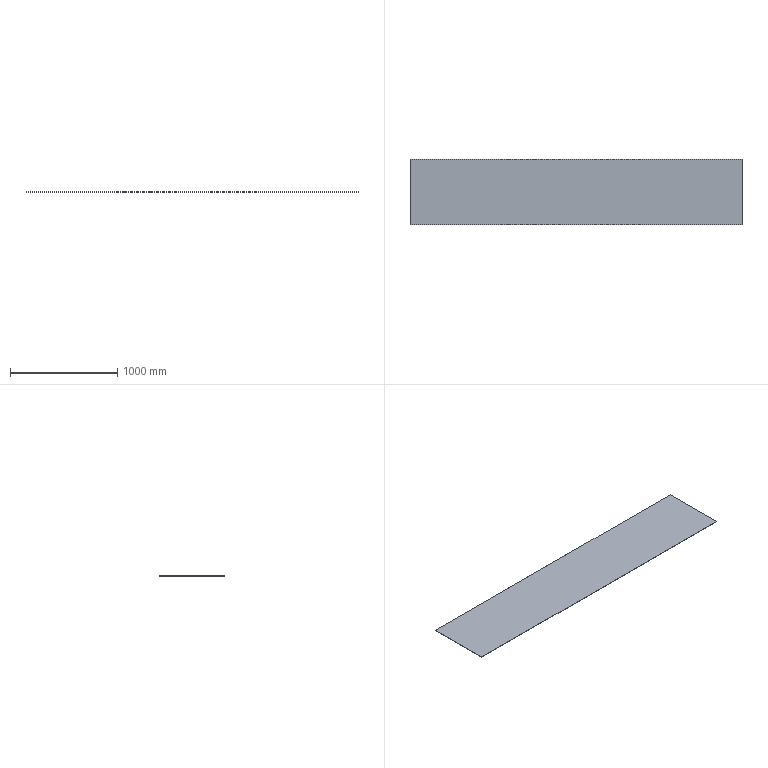Part | STEP file | 750038395 | 1 solid | 6 faces | box 3095 x 610 x 3 mm | volume 5663850 mm3 | plane 6
STEP:
#1=CARTESIAN_POINT('',(0.,-305.,3.));
#2=VERTEX_POINT('',#1);
#3=CARTESIAN_POINT('',(3095.,-305.,3.));
#4=VERTEX_POINT('',#3);
#5=CARTESIAN_POINT('',(0.,-305.,3.));
#6=DIRECTION('',(1.,0.,0.));
#7=VECTOR('',#6,1000.);
#8=LINE('',#5,#7);
#9=EDGE_CURVE('',#2,#4,#8,.T.);
#10=ORIENTED_EDGE('',*,*,#9,.T.);
#11=CARTESIAN_POINT('',(3095.,305.,3.));
#12=VERTEX_POINT('',#11);
#13=CARTESIAN_POINT('',(3095.,0.,3.));
#14=DIRECTION('',(0.,1.,0.));
#15=VECTOR('',#14,1000.);
#16=LINE('',#13,#15);
#17=EDGE_CURVE('',#4,#12,#16,.T.);
#18=ORIENTED_EDGE('',*,*,#17,.T.);
#19=CARTESIAN_POINT('',(0.,305.,3.));
#20=VERTEX_POINT('',#19);
#21=CARTESIAN_POINT('',(0.,305.,3.));
#22=DIRECTION('',(-1.,0.,0.));
#23=VECTOR('',#22,1000.);
#24=LINE('',#21,#23);
#25=EDGE_CURVE('',#12,#20,#24,.T.);
#26=ORIENTED_EDGE('',*,*,#25,.T.);
#27=CARTESIAN_POINT('',(0.,0.,3.));
#28=DIRECTION('',(0.,-1.,0.));
#29=VECTOR('',#28,1000.);
#30=LINE('',#27,#29);
#31=EDGE_CURVE('',#20,#2,#30,.T.);
#32=ORIENTED_EDGE('',*,*,#31,.T.);
#33=EDGE_LOOP('',(#10,#18,#26,#32));
#34=FACE_OUTER_BOUND('',#33,.T.);
#35=CARTESIAN_POINT('',(0.,0.,3.));
#36=DIRECTION('',(0.,0.,1.));
#37=DIRECTION('',(1.,0.,0.));
#38=AXIS2_PLACEMENT_3D('',#35,#36,#37);
#39=PLANE('',#38);
#40=ADVANCED_FACE('',(#34),#39,.T.);
#41=CARTESIAN_POINT('',(3095.,305.,0.));
#42=VERTEX_POINT('',#41);
#43=CARTESIAN_POINT('',(3095.,305.,3.));
#44=DIRECTION('',(0.,0.,-1.));
#45=VECTOR('',#44,1000.);
#46=LINE('',#43,#45);
#47=EDGE_CURVE('',#12,#42,#46,.T.);
#48=ORIENTED_EDGE('',*,*,#47,.F.);
#49=ORIENTED_EDGE('',*,*,#17,.F.);
#50=CARTESIAN_POINT('',(3095.,-305.,0.));
#51=VERTEX_POINT('',#50);
#52=CARTESIAN_POINT('',(3095.,-305.,3.));
#53=DIRECTION('',(0.,0.,1.));
#54=VECTOR('',#53,1000.);
#55=LINE('',#52,#54);
#56=EDGE_CURVE('',#51,#4,#55,.T.);
#57=ORIENTED_EDGE('',*,*,#56,.F.);
#58=CARTESIAN_POINT('',(3095.,-305.,0.));
#59=DIRECTION('',(0.,-1.,0.));
#60=VECTOR('',#59,1000.);
#61=LINE('',#58,#60);
#62=EDGE_CURVE('',#42,#51,#61,.T.);
#63=ORIENTED_EDGE('',*,*,#62,.F.);
#64=EDGE_LOOP('',(#48,#49,#57,#63));
#65=FACE_OUTER_BOUND('',#64,.T.);
#66=CARTESIAN_POINT('',(3095.,-305.,3.));
#67=DIRECTION('',(-1.,0.,0.));
#68=DIRECTION('',(0.,0.,1.));
#69=AXIS2_PLACEMENT_3D('',#66,#67,#68);
#70=PLANE('',#69);
#71=ADVANCED_FACE('',(#65),#70,.F.);
#72=ORIENTED_EDGE('',*,*,#56,.T.);
#73=ORIENTED_EDGE('',*,*,#9,.F.);
#74=CARTESIAN_POINT('',(0.,-305.,0.));
#75=VERTEX_POINT('',#74);
#76=CARTESIAN_POINT('',(0.,-305.,3.));
#77=DIRECTION('',(0.,0.,1.));
#78=VECTOR('',#77,1000.);
#79=LINE('',#76,#78);
#80=EDGE_CURVE('',#75,#2,#79,.T.);
#81=ORIENTED_EDGE('',*,*,#80,.F.);
#82=CARTESIAN_POINT('',(0.,-305.,0.));
#83=DIRECTION('',(-1.,0.,0.));
#84=VECTOR('',#83,1000.);
#85=LINE('',#82,#84);
#86=EDGE_CURVE('',#51,#75,#85,.T.);
#87=ORIENTED_EDGE('',*,*,#86,.F.);
#88=EDGE_LOOP('',(#72,#73,#81,#87));
#89=FACE_OUTER_BOUND('',#88,.T.);
#90=CARTESIAN_POINT('',(0.,-305.,3.));
#91=DIRECTION('',(0.,1.,0.));
#92=DIRECTION('',(0.,0.,1.));
#93=AXIS2_PLACEMENT_3D('',#90,#91,#92);
#94=PLANE('',#93);
#95=ADVANCED_FACE('',(#89),#94,.F.);
#96=ORIENTED_EDGE('',*,*,#80,.T.);
#97=ORIENTED_EDGE('',*,*,#31,.F.);
#98=CARTESIAN_POINT('',(0.,305.,0.));
#99=VERTEX_POINT('',#98);
#100=CARTESIAN_POINT('',(0.,305.,3.));
#101=DIRECTION('',(0.,0.,1.));
#102=VECTOR('',#101,1000.);
#103=LINE('',#100,#102);
#104=EDGE_CURVE('',#99,#20,#103,.T.);
#105=ORIENTED_EDGE('',*,*,#104,.F.);
#106=CARTESIAN_POINT('',(0.,305.,0.));
#107=DIRECTION('',(0.,1.,0.));
#108=VECTOR('',#107,1000.);
#109=LINE('',#106,#108);
#110=EDGE_CURVE('',#75,#99,#109,.T.);
#111=ORIENTED_EDGE('',*,*,#110,.F.);
#112=EDGE_LOOP('',(#96,#97,#105,#111));
#113=FACE_OUTER_BOUND('',#112,.T.);
#114=CARTESIAN_POINT('',(0.,305.,3.));
#115=DIRECTION('',(1.,0.,0.));
#116=DIRECTION('',(0.,0.,-1.));
#117=AXIS2_PLACEMENT_3D('',#114,#115,#116);
#118=PLANE('',#117);
#119=ADVANCED_FACE('',(#113),#118,.F.);
#120=ORIENTED_EDGE('',*,*,#104,.T.);
#121=ORIENTED_EDGE('',*,*,#25,.F.);
#122=ORIENTED_EDGE('',*,*,#47,.T.);
#123=CARTESIAN_POINT('',(3095.,305.,0.));
#124=DIRECTION('',(1.,0.,0.));
#125=VECTOR('',#124,1000.);
#126=LINE('',#123,#125);
#127=EDGE_CURVE('',#99,#42,#126,.T.);
#128=ORIENTED_EDGE('',*,*,#127,.F.);
#129=EDGE_LOOP('',(#120,#121,#122,#128));
#130=FACE_OUTER_BOUND('',#129,.T.);
#131=CARTESIAN_POINT('',(3095.,305.,3.));
#132=DIRECTION('',(0.,-1.,0.));
#133=DIRECTION('',(0.,0.,-1.));
#134=AXIS2_PLACEMENT_3D('',#131,#132,#133);
#135=PLANE('',#134);
#136=ADVANCED_FACE('',(#130),#135,.F.);
#137=ORIENTED_EDGE('',*,*,#62,.T.);
#138=ORIENTED_EDGE('',*,*,#86,.T.);
#139=ORIENTED_EDGE('',*,*,#110,.T.);
#140=ORIENTED_EDGE('',*,*,#127,.T.);
#141=EDGE_LOOP('',(#137,#138,#139,#140));
#142=FACE_OUTER_BOUND('',#141,.T.);
#143=CARTESIAN_POINT('',(0.,0.,0.));
#144=DIRECTION('',(0.,0.,1.));
#145=DIRECTION('',(1.,0.,0.));
#146=AXIS2_PLACEMENT_3D('',#143,#144,#145);
#147=PLANE('',#146);
#148=ADVANCED_FACE('',(#142),#147,.F.);
#149=CLOSED_SHELL('',(#40,#71,#95,#119,#136,#148));
#150=MANIFOLD_SOLID_BREP('',#149);
#151=CARTESIAN_POINT('',(0.,0.,0.));
#152=DIRECTION('',(0.,0.,1.));
#153=DIRECTION('',(1.,0.,0.));
#154=AXIS2_PLACEMENT_3D('',#151,#152,#153);
#155=(LENGTH_UNIT()NAMED_UNIT(*)SI_UNIT(.MILLI.,.METRE.));
#156=UNCERTAINTY_MEASURE_WITH_UNIT(LENGTH_MEASURE(0.00001),#155,'','');
#157=(NAMED_UNIT(*)PLANE_ANGLE_UNIT()SI_UNIT($,.RADIAN.));
#158=(NAMED_UNIT(*)SI_UNIT($,.STERADIAN.)SOLID_ANGLE_UNIT());
#159=(GEOMETRIC_REPRESENTATION_CONTEXT(3)GLOBAL_UNCERTAINTY_ASSIGNED_CONTEXT((#156))GLOBAL_UNIT_ASSIGNED_CONTEXT((#155,#157,#158))REPRESENTATION_CONTEXT('',''));
#160=ADVANCED_BREP_SHAPE_REPRESENTATION('',(#150,#154),#159);